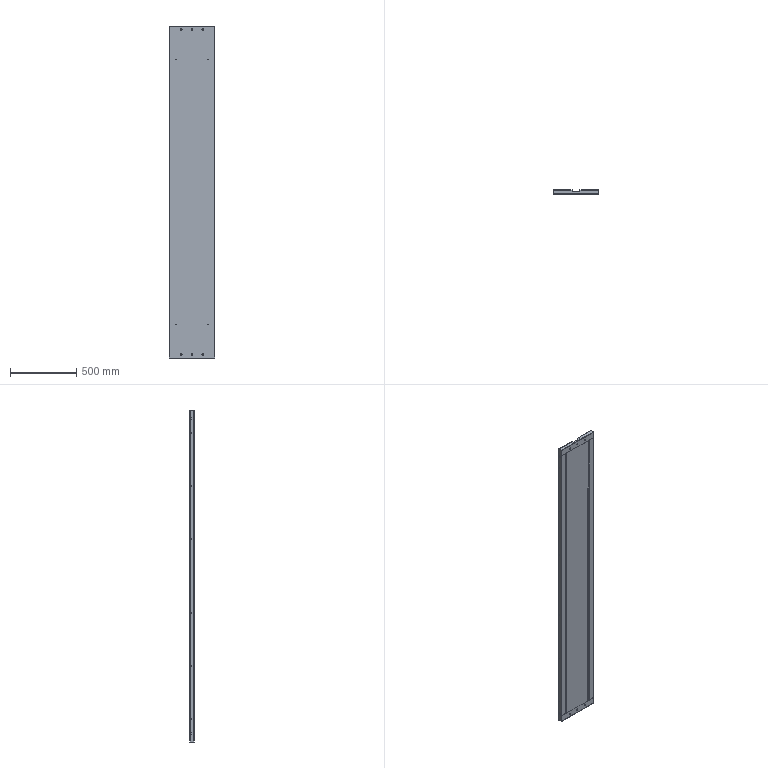Part | SolidWorks | features MirrorCompFeat 1, ReferencePattern 1 | 5 solids | 546 faces | box 346 x 32 x 2502 mm | volume 1579459 mm3 | plane 274 | cylinder 272 | commonest cylinder face diameters 6.2 x76 7 x76 5 x70 10.5 x24 2 x22 4 x4